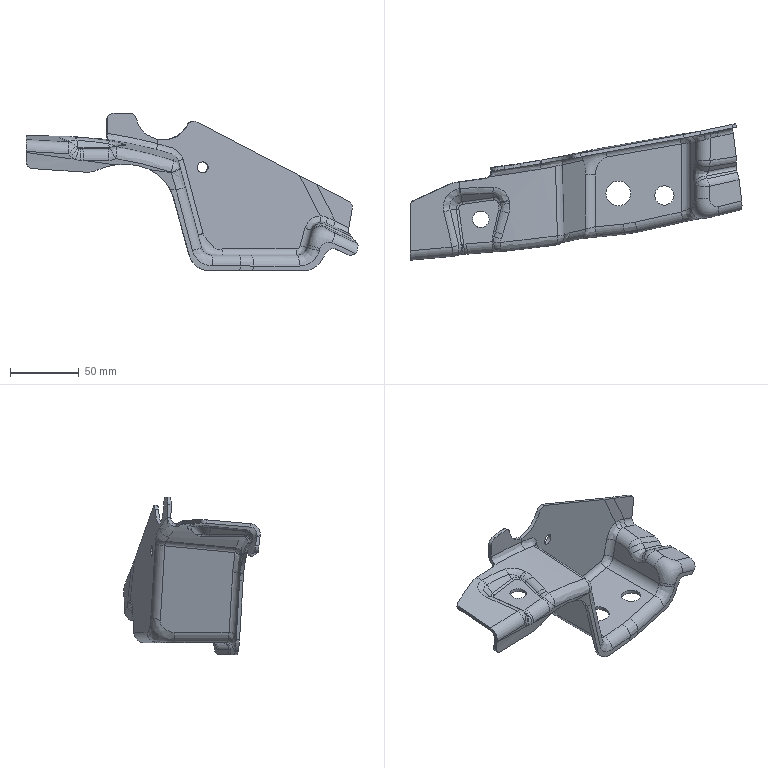Part | 1 solid | 249 faces | box 241.37 x 99.256 x 114.505 mm | volume 71590 mm3 | spline 142 | cylinder 68 | plane 23 | sphere 10 | other 6 | commonest cylinder face diameters 10 x20 15 x18 14 x6 5 x4 9 x4 12 x2